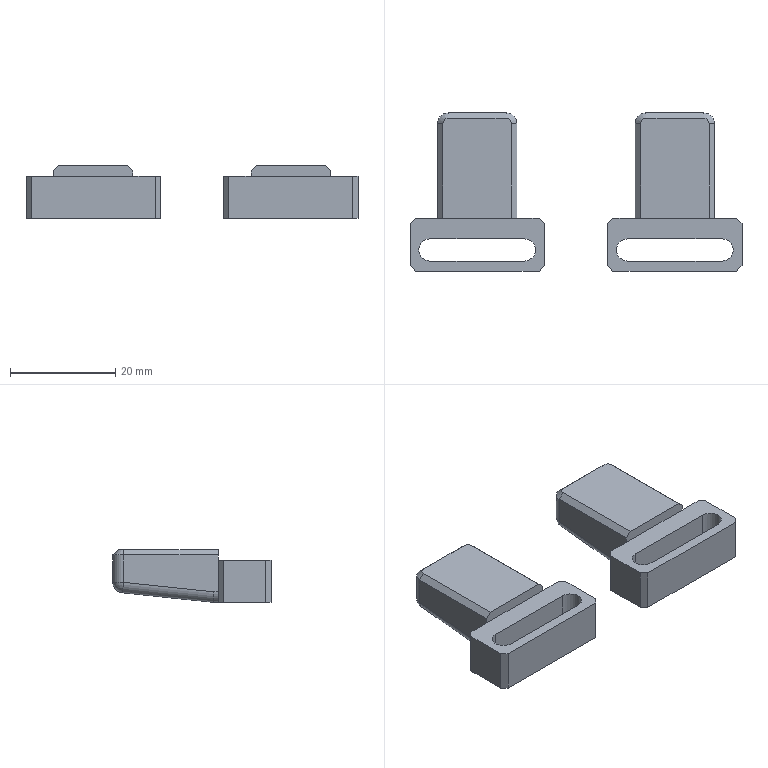NC program | NX | posted with a generic post | part box 63 x 30 x 10 mm
Whole program:
N10 G17 G21 G94 G90
(ZLEVEL_PROFILE_COPY_1_COPY_COPY_1_COPY , TOOL : D10JING)
N12 T14 M6
N14 G54
N16 G17 G0 G90 X-14.349 Y-9.544 B0. C0. S9500 M3
N18 G43 Z30. H14
N20 Z-17.17
N22 G94 G1 Z-18.17 F1000.
N24 X-13. Y-8.765
N26 G3 X-12.5 Y-7.899 R1.
N28 G1 Y-1. F1200.
N30 G3 X-13. Y-0.134 R1.
N32 G1 X-14.309 Y0.622
N34 Z-17.17
N36 G0 Z-14.255
N38 X-14.349 Y-9.64
N40 Z-18.085
N42 G1 Z-19.085 F1000.
N44 X-13. Y-8.861
N46 G3 X-12.5 Y-7.995 R1.
N48 G1 Y-1. F1200.
N50 G3 X-13. Y-0.134 R1.
N52 G1 X-14.309 Y0.622
N54 Z-18.085
N56 G0 Z30.
N58 X-3.817 Y-16.916
N60 Z-18.085
N62 G1 Z-19.085 F1000.
N64 X-4.634 Y-15.5
N66 G3 X-5.5 Y-15. R1.
N68 G2 X-11.697 Y-11.255 R7. F1200.
N70 G3 X-12.543 Y-10.721 R1.
N72 G1 X-14.098 Y-10.659
N74 Z-18.085
N76 G0 Z30.
N78 X-3.817 Y-16.916
N80 Z-19.
N82 G1 Z-20. F1000.
N84 X-4.634 Y-15.5
N86 G3 X-5.5 Y-15. R1.
N88 G2 X-12.5 Y-8. R7. F1200.
N90 G1 Y-1.
N92 G3 X-13. Y-0.134 R1.
N94 G1 X-14.309 Y0.622
N96 Z-19.
N98 G0 Z30.
N100 X14.309
N102 Z-17.17
N104 G1 Z-18.17 F1000.
N106 X13. Y-0.134
N108 G3 X12.5 Y-1. R1.
N110 G1 Y-7.899 F1200.
N112 G3 X13. Y-8.765 R1.
N114 G1 X14.349 Y-9.544
N116 Z-17.17
N118 G0 Z-14.255
N120 X14.309 Y0.622
N122 Z-18.085
N124 G1 Z-19.085 F1000.
N126 X13. Y-0.134
N128 G3 X12.5 Y-1. R1.
N130 G1 Y-7.995 F1200.
N132 G3 X13. Y-8.861 R1.
N134 G1 X14.349 Y-9.64
N136 Z-18.085
N138 G0 Z30.
N140 X14.102 Y-10.645
N142 Z-18.085
N144 G1 Z-19.085 F1000.
N146 X12.547 Y-10.71
N148 G3 X11.702 Y-11.245 R1.
N150 G2 X5.5 Y-15. R7. F1200.
N152 G3 X4.634 Y-15.5 R1.
N154 G1 X3.817 Y-16.916
N156 Z-18.085
N158 G0 Z30.
N160 X14.309 Y0.622
N162 Z-19.
N164 G1 Z-20. F1000.
N166 X13. Y-0.134
N168 G3 X12.5 Y-1. R1.
N170 G1 Y-8. F1200.
N172 G2 X5.5 Y-15. R7.
N174 G3 X4.634 Y-15.5 R1.
N176 G1 X3.817 Y-16.916
N178 Z-19.
N180 G0 Z30.
N182 M5
(HOLE_MILLING , TOOL : D6)
N184 T06 M6
N186 G54
N188 G17 G0 G90 X0. Y-11. B0. C0. S9500 M3
N190 G43 Z30. H6
N192 Z0.5
N194 G94 G3 X1. Y-12. R1. F1250.
N196 X2. Y-11. R1.
N198 X2. Y-11. Z-0.5 I-2. J0.
N200 X2. Y-11. Z-1.5 I-2. J0.
N202 X2. Y-11. Z-2.5 I-2. J0.
N204 X2. Y-11. Z-3.5 I-2. J0.
N206 X2. Y-11. Z-4.5 I-2. J0.
N208 X2. Y-11. Z-5.5 I-2. J0.
N210 X2. Y-11. Z-6.5 I-2. J0.
N212 X2. Y-11. Z-7.5 I-2. J0.
N214 X2. Y-11. Z-8.5 I-2. J0.
N216 X2. Y-11. Z-9.5 I-2. J0.
N218 X2. Y-11. Z-10.5 I-2. J0.
N220 X2. Y-11. Z-11.5 I-2. J0.
N222 X2. Y-11. Z-12.5 I-2. J0.
N224 X2. Y-11. Z-13.5 I-2. J0.
N226 X2. Y-11. Z-14.5 I-2. J0.
N228 X2. Y-11. Z-15.5 I-2. J0.
N230 X2. Y-11. Z-16.5 I-2. J0.
N232 X2. Y-11. Z-17.5 I-2. J0.
N234 X2. Y-11. Z-18.5 I-2. J0.
N236 X2. Y-11. Z-19.5 I-2. J0.
N238 X-2. Y-11. Z-20. I-2. J0.
N240 X0. Y-13. R2.
N242 X-2. Y-11. R-2.
N244 X-1. Y-12. R1.
N246 X0. Y-11. R1.
N248 G0 Z30.
N250 M5
N252 M2